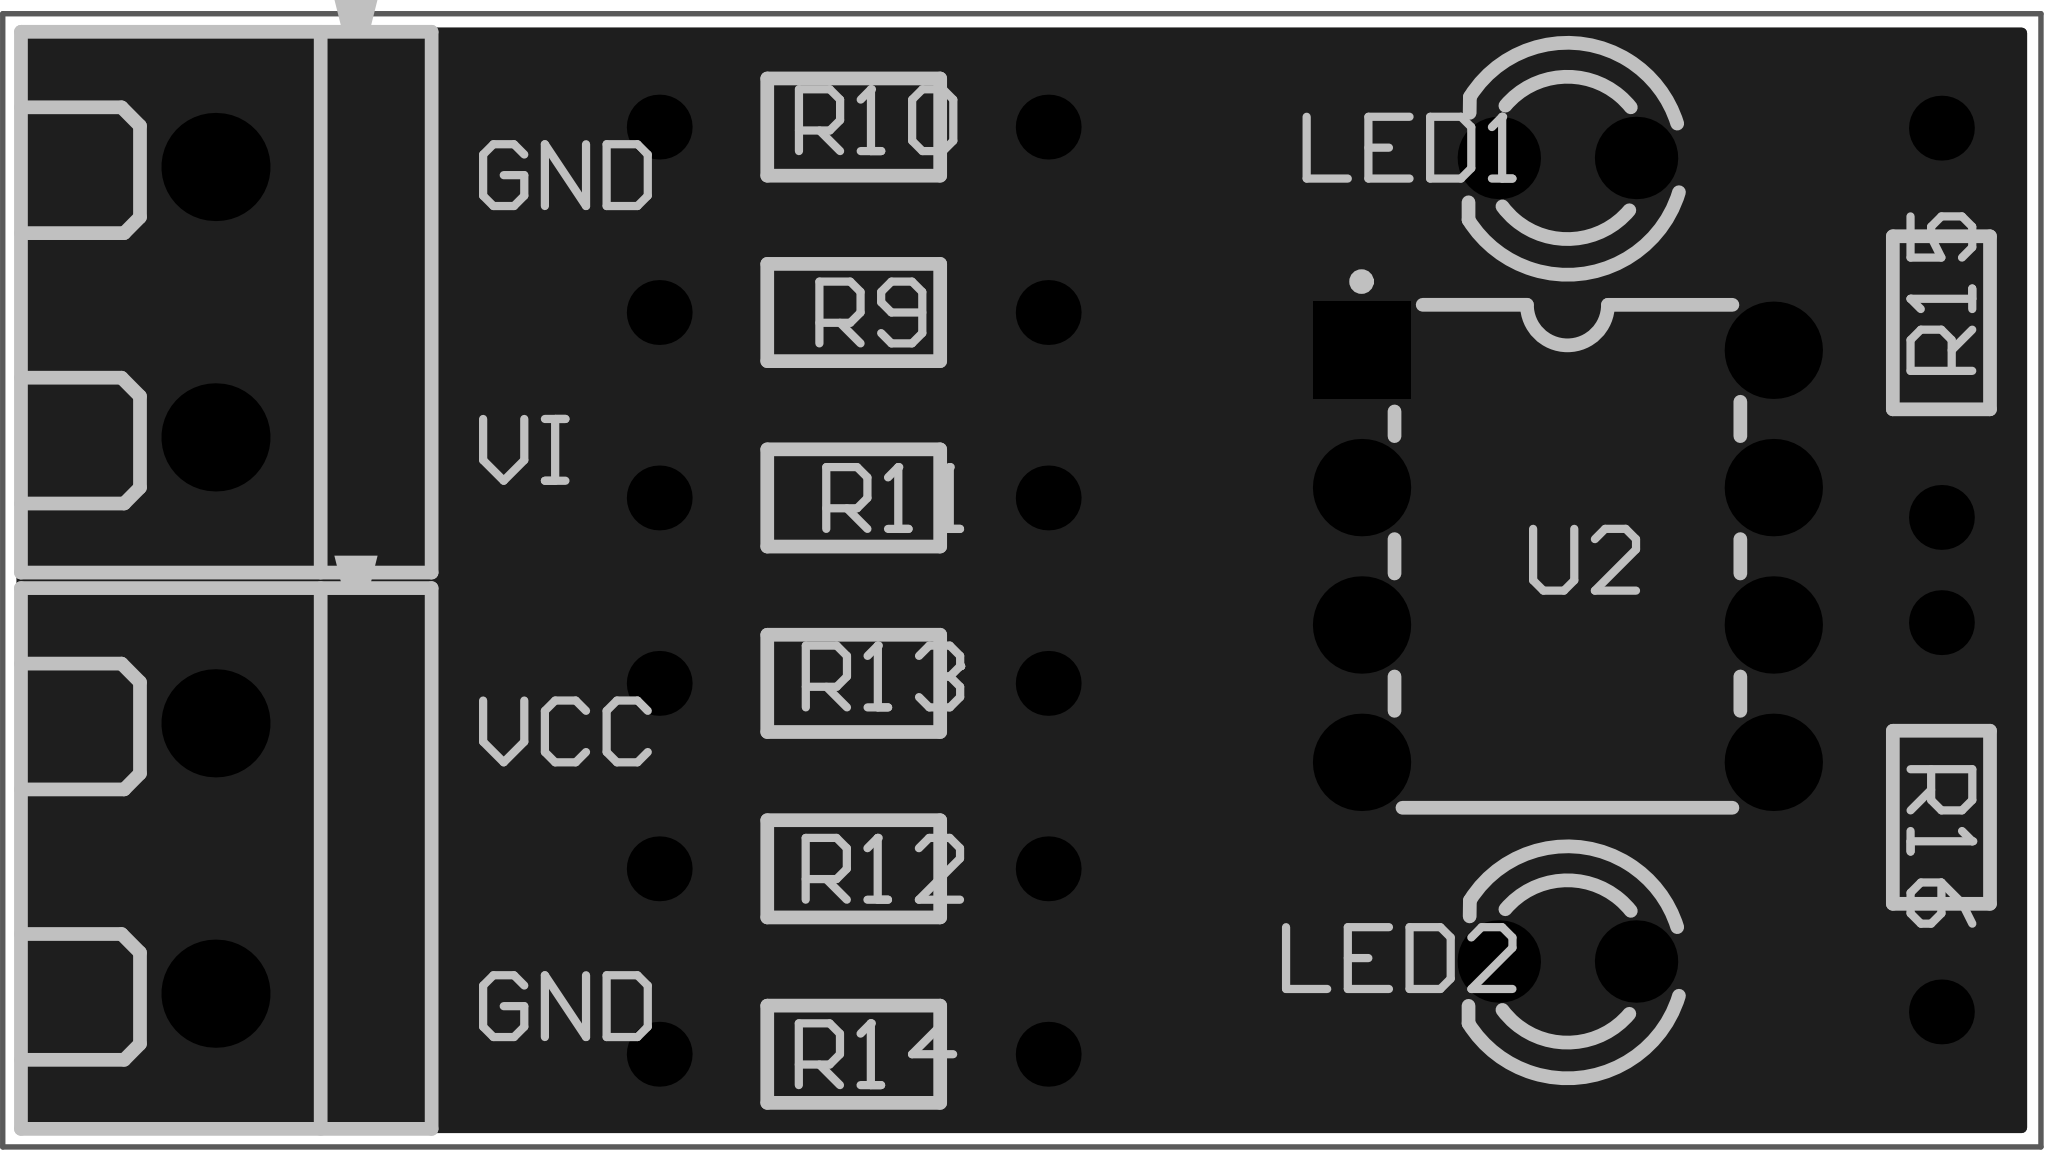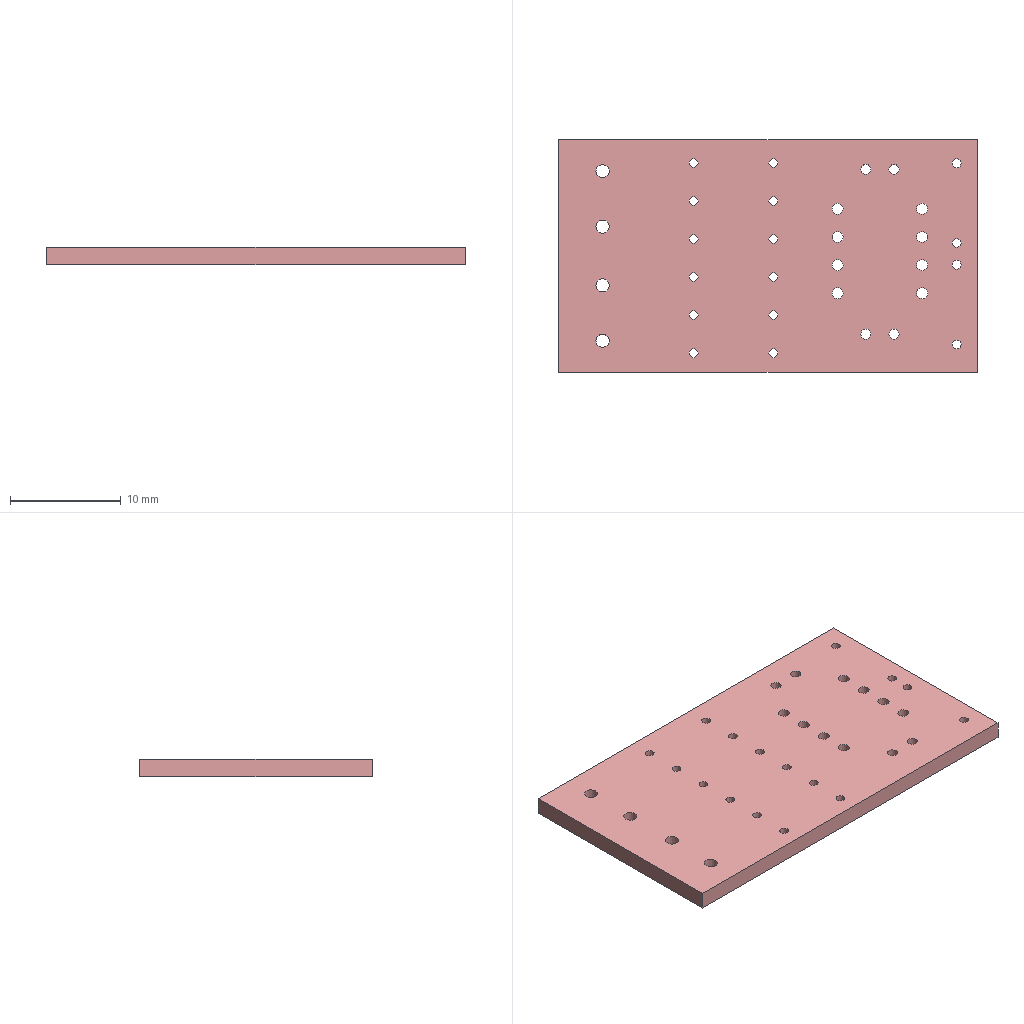Circuit board layout | Altium Designer | box 37.7 x 21 x 1.6 mm
Layer stack:
# Altium Designer layer stack of  (unit mm; dielectric type: 0 none, 1 core, 2 prepreg, 3 surface material)
index,name,kind,layer,copper_thickness_mm,dielectric_type,dielectric_thickness_mm,dielectric_material,dielectric_constant
0,Top Paste Mask Layer,other,,,,,,
1,Top Silkscreen Layer,other,,,,,,
2,Top Solder Mask Layer,dielectric,,,3,0.01,,3.3
3,Top Layer,copper,Top Layer,0.035,,,,
4,Dielectric1,dielectric,,,3,1.51,FR4,4.5
5,Bottom Layer,copper,Bottom Layer,0.035,,,,
6,Bottom Solder Mask Layer,dielectric,,,3,0.01,,3.3
7,Bottom Silkscreen Layer,other,,,,,,
8,Bottom Paste Mask Layer,other,,,,,,
# drill layer pairs: low layer,high layer
drill_pair,Top Layer,Bottom Layer
Part placement:
Designator,Comment,Layer,Footprint,Center-X(mm),Center-Y(mm),Rotation
P1,KF301-2P接线端子,TopLayer,CONN-TH_XY301V-A-5.0-2P,83.058,84.709,90
P2,KF301-2P接线端子,TopLayer,CONN-TH_XY301V-A-5.0-2P,83.058,94.996,90
LED1,,TopLayer,LED_TH-3mm,108.077,97.663,180
LED2,,TopLayer,LED_TH-3mm,108.077,82.804,180
R9,30K,TopLayer,Res_1/8W,94.869,94.805,0
R10,68K,TopLayer,Res_1/8W,94.869,98.234,0
R11,30K,TopLayer,Res_1/8W,94.869,91.376,180
R12,68K,TopLayer,Res_1/8W,94.869,84.518,0
R13,51K,TopLayer,Res_1/8W,94.869,87.947,0
R14,13K,TopLayer,Res_1/8W,94.869,81.089,0
R15,220,TopLayer,Res_1/8W,114.998,94.615,90
R16,220,TopLayer,Res_1/8W,114.998,85.471,270
U2,LM324AD,TopLayer,DIP-8_L9.3-W6.4-P2.54-LS7.6-BL,108.077,90.297,270
Pad and via stacks:
# Altium Designer via and pad stacks of  (unit mm). Each distinct definition once, with the count of objects using it.
# via: kind,start_layer,end_layer,hole_mm,diameter_mm,mode(0 simple;1 top-mid-bottom;2 full stack),diameter_per_layer,count,example_net
# pad: kind,layer,hole_mm,hole_type(0 round;1 square;2 slot),plating,top_size,top_shape(1 round;2 rect;3 octagon;9 rounded rect),mid_size,bottom_size,mode,footprint,size_per_layer,count,example
pad,Multi-Layer,1.2,0,plated,2x2,1,2x2,2x2,0,CONN-TH_XY301V-A-5.0-2P,,4,P1.1
pad,Multi-Layer,0.9144,0,plated,1.524x1.524,1,1.524x1.524,1.524x1.524,0,LED_TH-3mm,,4,LED1.1
pad,Multi-Layer,0.8001,0,plated,1.199x1.199,1,1.199x1.199,1.199x1.199,0,Res_1/8W,,16,R9.1
pad,Multi-Layer,1,0,plated,1.8x1.8,2,1.8x1.8,1.8x1.8,0,DIP-8_L9.3-W6.4-P2.54-LS7.6-BL,,1,U2.1
pad,Multi-Layer,1,0,plated,1.8x1.8,1,1.8x1.8,1.8x1.8,0,DIP-8_L9.3-W6.4-P2.54-LS7.6-BL,,7,U2.2
Copper pours:
name,layer,net,type(0 solid;1 hatched;2 none)
Bottom Layer-GND,Bottom Layer,GND,0
Top Layer-GND,Top Layer,GND,0